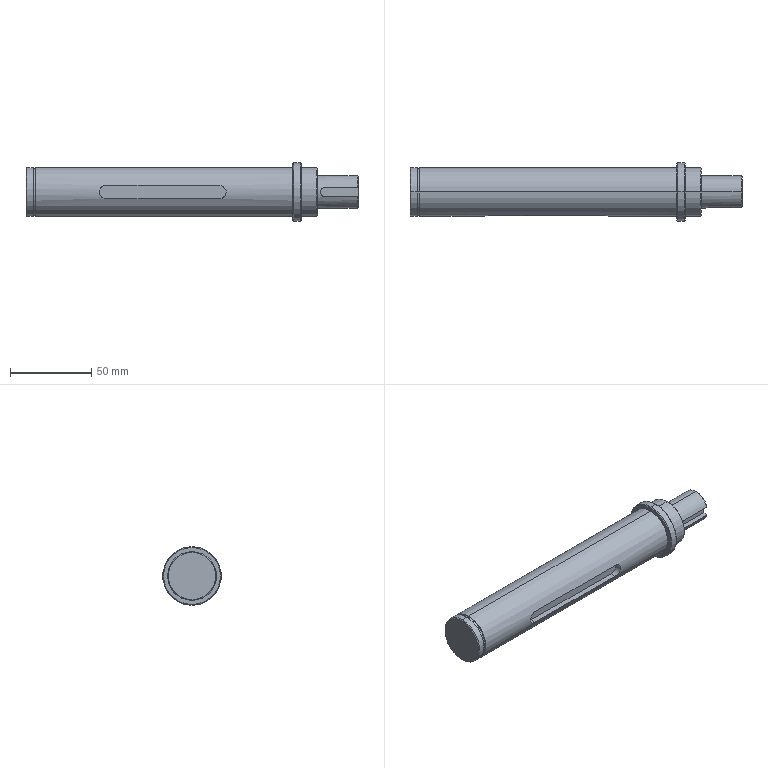Part | SolidWorks | features ICE 2, Chamfer 1, Revolution 1 | 1 solid | 39 faces | box 204 x 36 x 36 mm | volume 132992 mm3 | cylinder 15 | plane 13 | cone 11 | commonest cylinder face diameters 30 x6 8 x2 20 x2 28.6 x2 36 x2 6 x1
STEP:
#1=CARTESIAN_POINT('',(0.,0.,14.5));
#2=VERTEX_POINT('',#1);
#3=CARTESIAN_POINT('',(0.,0.,-14.5));
#4=VERTEX_POINT('',#3);
#5=CARTESIAN_POINT('',(0.,0.,0.));
#6=DIRECTION('',(-1.,0.,0.));
#7=DIRECTION('',(0.,0.,-1.));
#8=AXIS2_PLACEMENT_3D('',#5,#6,#7);
#9=CIRCLE('',#8,14.5);
#10=EDGE_CURVE('',#2,#4,#9,.T.);
#11=ORIENTED_EDGE('',*,*,#10,.F.);
#12=CARTESIAN_POINT('',(0.5,0.,15.));
#13=VERTEX_POINT('',#12);
#14=CARTESIAN_POINT('',(0.,0.,14.5));
#15=DIRECTION('',(0.7071,0.,0.7071));
#16=VECTOR('',#15,1000.);
#17=LINE('',#14,#16);
#18=EDGE_CURVE('',#2,#13,#17,.T.);
#19=ORIENTED_EDGE('',*,*,#18,.T.);
#20=CARTESIAN_POINT('',(0.5,0.,-15.));
#21=VERTEX_POINT('',#20);
#22=CARTESIAN_POINT('',(0.5,0.,0.));
#23=DIRECTION('',(1.,0.,0.));
#24=DIRECTION('',(0.,0.,-1.));
#25=AXIS2_PLACEMENT_3D('',#22,#23,#24);
#26=CIRCLE('',#25,15.);
#27=EDGE_CURVE('',#21,#13,#26,.T.);
#28=ORIENTED_EDGE('',*,*,#27,.F.);
#29=CARTESIAN_POINT('',(0.,0.,-14.5));
#30=DIRECTION('',(0.7071,0.,-0.7071));
#31=VECTOR('',#30,1000.);
#32=LINE('',#29,#31);
#33=EDGE_CURVE('',#4,#21,#32,.T.);
#34=ORIENTED_EDGE('',*,*,#33,.F.);
#35=EDGE_LOOP('',(#11,#19,#28,#34));
#36=FACE_OUTER_BOUND('',#35,.T.);
#37=CARTESIAN_POINT('',(0.,0.,0.));
#38=DIRECTION('',(1.,0.,0.));
#39=DIRECTION('',(0.,0.,-1.));
#40=AXIS2_PLACEMENT_3D('',#37,#38,#39);
#41=CONICAL_SURFACE('',#40,14.5,0.7854);
#42=ADVANCED_FACE('',(#36),#41,.T.);
#43=CARTESIAN_POINT('',(169.,0.,-17.5));
#44=VERTEX_POINT('',#43);
#45=CARTESIAN_POINT('',(169.,0.,17.5));
#46=VERTEX_POINT('',#45);
#47=CARTESIAN_POINT('',(169.,0.,0.));
#48=DIRECTION('',(1.,0.,0.));
#49=DIRECTION('',(0.,0.,1.));
#50=AXIS2_PLACEMENT_3D('',#47,#48,#49);
#51=CIRCLE('',#50,17.5);
#52=EDGE_CURVE('',#44,#46,#51,.T.);
#53=ORIENTED_EDGE('',*,*,#52,.F.);
#54=CARTESIAN_POINT('',(168.5,0.,-18.));
#55=VERTEX_POINT('',#54);
#56=CARTESIAN_POINT('',(168.5,0.,-18.));
#57=DIRECTION('',(-0.7071,0.,-0.7071));
#58=VECTOR('',#57,1000.);
#59=LINE('',#56,#58);
#60=EDGE_CURVE('',#44,#55,#59,.T.);
#61=ORIENTED_EDGE('',*,*,#60,.T.);
#62=CARTESIAN_POINT('',(168.5,0.,18.));
#63=VERTEX_POINT('',#62);
#64=CARTESIAN_POINT('',(168.5,0.,0.));
#65=DIRECTION('',(-1.,0.,0.));
#66=DIRECTION('',(0.,0.,1.));
#67=AXIS2_PLACEMENT_3D('',#64,#65,#66);
#68=CIRCLE('',#67,18.);
#69=EDGE_CURVE('',#63,#55,#68,.T.);
#70=ORIENTED_EDGE('',*,*,#69,.F.);
#71=CARTESIAN_POINT('',(168.5,0.,18.));
#72=DIRECTION('',(-0.7071,0.,0.7071));
#73=VECTOR('',#72,1000.);
#74=LINE('',#71,#73);
#75=EDGE_CURVE('',#46,#63,#74,.T.);
#76=ORIENTED_EDGE('',*,*,#75,.F.);
#77=EDGE_LOOP('',(#53,#61,#70,#76));
#78=FACE_OUTER_BOUND('',#77,.T.);
#79=CARTESIAN_POINT('',(168.5,0.,0.));
#80=DIRECTION('',(-1.,0.,0.));
#81=DIRECTION('',(0.,0.,1.));
#82=AXIS2_PLACEMENT_3D('',#79,#80,#81);
#83=CONICAL_SURFACE('',#82,18.,0.7854);
#84=ADVANCED_FACE('',(#78),#83,.T.);
#85=CARTESIAN_POINT('',(164.,0.,17.5));
#86=VERTEX_POINT('',#85);
#87=CARTESIAN_POINT('',(164.,0.,-17.5));
#88=VERTEX_POINT('',#87);
#89=CARTESIAN_POINT('',(164.,0.,0.));
#90=DIRECTION('',(-1.,0.,0.));
#91=DIRECTION('',(0.,0.,-1.));
#92=AXIS2_PLACEMENT_3D('',#89,#90,#91);
#93=CIRCLE('',#92,17.5);
#94=EDGE_CURVE('',#86,#88,#93,.T.);
#95=ORIENTED_EDGE('',*,*,#94,.F.);
#96=CARTESIAN_POINT('',(164.5,0.,18.));
#97=VERTEX_POINT('',#96);
#98=CARTESIAN_POINT('',(164.,0.,17.5));
#99=DIRECTION('',(0.7071,0.,0.7071));
#100=VECTOR('',#99,1000.);
#101=LINE('',#98,#100);
#102=EDGE_CURVE('',#86,#97,#101,.T.);
#103=ORIENTED_EDGE('',*,*,#102,.T.);
#104=CARTESIAN_POINT('',(164.5,0.,-18.));
#105=VERTEX_POINT('',#104);
#106=CARTESIAN_POINT('',(164.5,0.,0.));
#107=DIRECTION('',(1.,0.,0.));
#108=DIRECTION('',(0.,0.,-1.));
#109=AXIS2_PLACEMENT_3D('',#106,#107,#108);
#110=CIRCLE('',#109,18.);
#111=EDGE_CURVE('',#105,#97,#110,.T.);
#112=ORIENTED_EDGE('',*,*,#111,.F.);
#113=CARTESIAN_POINT('',(164.,0.,-17.5));
#114=DIRECTION('',(0.7071,0.,-0.7071));
#115=VECTOR('',#114,1000.);
#116=LINE('',#113,#115);
#117=EDGE_CURVE('',#88,#105,#116,.T.);
#118=ORIENTED_EDGE('',*,*,#117,.F.);
#119=EDGE_LOOP('',(#95,#103,#112,#118));
#120=FACE_OUTER_BOUND('',#119,.T.);
#121=CARTESIAN_POINT('',(164.,0.,0.));
#122=DIRECTION('',(1.,0.,0.));
#123=DIRECTION('',(0.,0.,-1.));
#124=AXIS2_PLACEMENT_3D('',#121,#122,#123);
#125=CONICAL_SURFACE('',#124,17.5,0.7854);
#126=ADVANCED_FACE('',(#120),#125,.T.);
#127=CARTESIAN_POINT('',(179.,0.,-14.5));
#128=VERTEX_POINT('',#127);
#129=CARTESIAN_POINT('',(179.,0.,14.5));
#130=VERTEX_POINT('',#129);
#131=CARTESIAN_POINT('',(179.,0.,0.));
#132=DIRECTION('',(1.,0.,0.));
#133=DIRECTION('',(0.,0.,1.));
#134=AXIS2_PLACEMENT_3D('',#131,#132,#133);
#135=CIRCLE('',#134,14.5);
#136=EDGE_CURVE('',#128,#130,#135,.T.);
#137=ORIENTED_EDGE('',*,*,#136,.F.);
#138=CARTESIAN_POINT('',(178.5,0.,-15.));
#139=VERTEX_POINT('',#138);
#140=CARTESIAN_POINT('',(178.5,0.,-15.));
#141=DIRECTION('',(-0.7071,0.,-0.7071));
#142=VECTOR('',#141,1000.);
#143=LINE('',#140,#142);
#144=EDGE_CURVE('',#128,#139,#143,.T.);
#145=ORIENTED_EDGE('',*,*,#144,.T.);
#146=CARTESIAN_POINT('',(178.5,0.,15.));
#147=VERTEX_POINT('',#146);
#148=CARTESIAN_POINT('',(178.5,0.,0.));
#149=DIRECTION('',(-1.,0.,0.));
#150=DIRECTION('',(0.,0.,1.));
#151=AXIS2_PLACEMENT_3D('',#148,#149,#150);
#152=CIRCLE('',#151,15.);
#153=EDGE_CURVE('',#147,#139,#152,.T.);
#154=ORIENTED_EDGE('',*,*,#153,.F.);
#155=CARTESIAN_POINT('',(178.5,0.,15.));
#156=DIRECTION('',(-0.7071,0.,0.7071));
#157=VECTOR('',#156,1000.);
#158=LINE('',#155,#157);
#159=EDGE_CURVE('',#130,#147,#158,.T.);
#160=ORIENTED_EDGE('',*,*,#159,.F.);
#161=EDGE_LOOP('',(#137,#145,#154,#160));
#162=FACE_OUTER_BOUND('',#161,.T.);
#163=CARTESIAN_POINT('',(178.5,0.,0.));
#164=DIRECTION('',(-1.,0.,0.));
#165=DIRECTION('',(0.,0.,1.));
#166=AXIS2_PLACEMENT_3D('',#163,#164,#165);
#167=CONICAL_SURFACE('',#166,15.,0.7854);
#168=ADVANCED_FACE('',(#162),#167,.T.);
#169=CARTESIAN_POINT('',(204.,0.,-9.5));
#170=VERTEX_POINT('',#169);
#171=CARTESIAN_POINT('',(204.,0.,9.5));
#172=VERTEX_POINT('',#171);
#173=CARTESIAN_POINT('',(204.,0.,0.));
#174=DIRECTION('',(1.,0.,0.));
#175=DIRECTION('',(0.,0.,1.));
#176=AXIS2_PLACEMENT_3D('',#173,#174,#175);
#177=CIRCLE('',#176,9.5);
#178=EDGE_CURVE('',#170,#172,#177,.T.);
#179=ORIENTED_EDGE('',*,*,#178,.F.);
#180=CARTESIAN_POINT('',(203.5,0.,-10.));
#181=VERTEX_POINT('',#180);
#182=CARTESIAN_POINT('',(203.5,0.,-10.));
#183=DIRECTION('',(-0.7071,0.,-0.7071));
#184=VECTOR('',#183,1000.);
#185=LINE('',#182,#184);
#186=EDGE_CURVE('',#170,#181,#185,.T.);
#187=ORIENTED_EDGE('',*,*,#186,.T.);
#188=CARTESIAN_POINT('',(203.5,0.,10.));
#189=VERTEX_POINT('',#188);
#190=CARTESIAN_POINT('',(203.5,0.,0.));
#191=DIRECTION('',(-1.,0.,0.));
#192=DIRECTION('',(0.,0.,1.));
#193=AXIS2_PLACEMENT_3D('',#190,#191,#192);
#194=CIRCLE('',#193,10.);
#195=EDGE_CURVE('',#189,#181,#194,.T.);
#196=ORIENTED_EDGE('',*,*,#195,.F.);
#197=CARTESIAN_POINT('',(203.5,0.,10.));
#198=DIRECTION('',(-0.7071,0.,0.7071));
#199=VECTOR('',#198,1000.);
#200=LINE('',#197,#199);
#201=EDGE_CURVE('',#172,#189,#200,.T.);
#202=ORIENTED_EDGE('',*,*,#201,.F.);
#203=EDGE_LOOP('',(#179,#187,#196,#202));
#204=FACE_OUTER_BOUND('',#203,.T.);
#205=CARTESIAN_POINT('',(203.5,0.,0.));
#206=DIRECTION('',(-1.,0.,0.));
#207=DIRECTION('',(0.,0.,1.));
#208=AXIS2_PLACEMENT_3D('',#205,#206,#207);
#209=CONICAL_SURFACE('',#208,10.,0.7854);
#210=ADVANCED_FACE('',(#204),#209,.T.);
#211=CARTESIAN_POINT('',(204.,-9.014,3.));
#212=VERTEX_POINT('',#211);
#213=CARTESIAN_POINT('',(204.,0.,0.));
#214=DIRECTION('',(1.,0.,0.));
#215=DIRECTION('',(0.,0.,1.));
#216=AXIS2_PLACEMENT_3D('',#213,#214,#215);
#217=CIRCLE('',#216,9.5);
#218=EDGE_CURVE('',#172,#212,#217,.T.);
#219=ORIENTED_EDGE('',*,*,#218,.F.);
#220=ORIENTED_EDGE('',*,*,#201,.T.);
#221=CARTESIAN_POINT('',(203.5,-9.539,3.));
#222=VERTEX_POINT('',#221);
#223=CARTESIAN_POINT('',(203.5,0.,0.));
#224=DIRECTION('',(-1.,0.,0.));
#225=DIRECTION('',(0.,0.,1.));
#226=AXIS2_PLACEMENT_3D('',#223,#224,#225);
#227=CIRCLE('',#226,10.);
#228=EDGE_CURVE('',#222,#189,#227,.T.);
#229=ORIENTED_EDGE('',*,*,#228,.F.);
#230=CARTESIAN_POINT('',(204.,-9.014,3.));
#231=CARTESIAN_POINT('',(203.834,-9.189,3.));
#232=CARTESIAN_POINT('',(203.667,-9.364,3.));
#233=CARTESIAN_POINT('',(203.5,-9.539,3.));
#234=B_SPLINE_CURVE_WITH_KNOTS('',3,(#230,#231,#232,#233),.UNSPECIFIED.,.F.,.F.,(4,4),(0.005234,0.005959),.UNSPECIFIED.);
#235=EDGE_CURVE('',#212,#222,#234,.T.);
#236=ORIENTED_EDGE('',*,*,#235,.F.);
#237=EDGE_LOOP('',(#219,#220,#229,#236));
#238=FACE_OUTER_BOUND('',#237,.T.);
#239=CARTESIAN_POINT('',(203.5,0.,0.));
#240=DIRECTION('',(-1.,0.,0.));
#241=DIRECTION('',(0.,0.,1.));
#242=AXIS2_PLACEMENT_3D('',#239,#240,#241);
#243=CONICAL_SURFACE('',#242,10.,0.7854);
#244=ADVANCED_FACE('',(#238),#243,.T.);
#245=ORIENTED_EDGE('',*,*,#195,.T.);
#246=CARTESIAN_POINT('',(179.,0.,-10.));
#247=VERTEX_POINT('',#246);
#248=CARTESIAN_POINT('',(0.,0.,-10.));
#249=DIRECTION('',(-1.,0.,0.));
#250=VECTOR('',#249,1000.);
#251=LINE('',#248,#250);
#252=EDGE_CURVE('',#181,#247,#251,.T.);
#253=ORIENTED_EDGE('',*,*,#252,.T.);
#254=CARTESIAN_POINT('',(179.,0.,10.));
#255=VERTEX_POINT('',#254);
#256=CARTESIAN_POINT('',(179.,0.,0.));
#257=DIRECTION('',(-1.,0.,0.));
#258=DIRECTION('',(0.,0.,1.));
#259=AXIS2_PLACEMENT_3D('',#256,#257,#258);
#260=CIRCLE('',#259,10.);
#261=EDGE_CURVE('',#255,#247,#260,.T.);
#262=ORIENTED_EDGE('',*,*,#261,.F.);
#263=CARTESIAN_POINT('',(0.,0.,10.));
#264=DIRECTION('',(-1.,0.,0.));
#265=VECTOR('',#264,1000.);
#266=LINE('',#263,#265);
#267=EDGE_CURVE('',#189,#255,#266,.T.);
#268=ORIENTED_EDGE('',*,*,#267,.F.);
#269=EDGE_LOOP('',(#245,#253,#262,#268));
#270=FACE_OUTER_BOUND('',#269,.T.);
#271=CARTESIAN_POINT('',(0.,0.,0.));
#272=DIRECTION('',(-1.,0.,0.));
#273=DIRECTION('',(0.,0.,1.));
#274=AXIS2_PLACEMENT_3D('',#271,#272,#273);
#275=CYLINDRICAL_SURFACE('',#274,10.);
#276=ADVANCED_FACE('',(#270),#275,.T.);
#277=ORIENTED_EDGE('',*,*,#153,.T.);
#278=CARTESIAN_POINT('',(169.,0.,-15.));
#279=VERTEX_POINT('',#278);
#280=CARTESIAN_POINT('',(0.,0.,-15.));
#281=DIRECTION('',(-1.,0.,0.));
#282=VECTOR('',#281,1000.);
#283=LINE('',#280,#282);
#284=EDGE_CURVE('',#139,#279,#283,.T.);
#285=ORIENTED_EDGE('',*,*,#284,.T.);
#286=CARTESIAN_POINT('',(169.,0.,15.));
#287=VERTEX_POINT('',#286);
#288=CARTESIAN_POINT('',(169.,0.,0.));
#289=DIRECTION('',(-1.,0.,0.));
#290=DIRECTION('',(0.,0.,1.));
#291=AXIS2_PLACEMENT_3D('',#288,#289,#290);
#292=CIRCLE('',#291,15.);
#293=EDGE_CURVE('',#287,#279,#292,.T.);
#294=ORIENTED_EDGE('',*,*,#293,.F.);
#295=CARTESIAN_POINT('',(0.,0.,15.));
#296=DIRECTION('',(-1.,0.,0.));
#297=VECTOR('',#296,1000.);
#298=LINE('',#295,#297);
#299=EDGE_CURVE('',#147,#287,#298,.T.);
#300=ORIENTED_EDGE('',*,*,#299,.F.);
#301=EDGE_LOOP('',(#277,#285,#294,#300));
#302=FACE_OUTER_BOUND('',#301,.T.);
#303=CARTESIAN_POINT('',(0.,0.,0.));
#304=DIRECTION('',(-1.,0.,0.));
#305=DIRECTION('',(0.,0.,1.));
#306=AXIS2_PLACEMENT_3D('',#303,#304,#305);
#307=CYLINDRICAL_SURFACE('',#306,15.);
#308=ADVANCED_FACE('',(#302),#307,.T.);
#309=ORIENTED_EDGE('',*,*,#69,.T.);
#310=CARTESIAN_POINT('',(0.,0.,-18.));
#311=DIRECTION('',(-1.,0.,0.));
#312=VECTOR('',#311,1000.);
#313=LINE('',#310,#312);
#314=EDGE_CURVE('',#55,#105,#313,.T.);
#315=ORIENTED_EDGE('',*,*,#314,.T.);
#316=ORIENTED_EDGE('',*,*,#111,.T.);
#317=CARTESIAN_POINT('',(0.,0.,18.));
#318=DIRECTION('',(-1.,0.,0.));
#319=VECTOR('',#318,1000.);
#320=LINE('',#317,#319);
#321=EDGE_CURVE('',#63,#97,#320,.T.);
#322=ORIENTED_EDGE('',*,*,#321,.F.);
#323=EDGE_LOOP('',(#309,#315,#316,#322));
#324=FACE_OUTER_BOUND('',#323,.T.);
#325=CARTESIAN_POINT('',(0.,0.,0.));
#326=DIRECTION('',(-1.,0.,0.));
#327=DIRECTION('',(0.,0.,1.));
#328=AXIS2_PLACEMENT_3D('',#325,#326,#327);
#329=CYLINDRICAL_SURFACE('',#328,18.);
#330=ADVANCED_FACE('',(#324),#329,.T.);
#331=CARTESIAN_POINT('',(164.,0.,15.));
#332=VERTEX_POINT('',#331);
#333=CARTESIAN_POINT('',(164.,0.,-15.));
#334=VERTEX_POINT('',#333);
#335=CARTESIAN_POINT('',(164.,0.,0.));
#336=DIRECTION('',(-1.,0.,0.));
#337=DIRECTION('',(0.,0.,1.));
#338=AXIS2_PLACEMENT_3D('',#335,#336,#337);
#339=CIRCLE('',#338,15.);
#340=EDGE_CURVE('',#332,#334,#339,.T.);
#341=ORIENTED_EDGE('',*,*,#340,.T.);
#342=CARTESIAN_POINT('',(6.,0.,-15.));
#343=VERTEX_POINT('',#342);
#344=CARTESIAN_POINT('',(0.,0.,-15.));
#345=DIRECTION('',(-1.,0.,0.));
#346=VECTOR('',#345,1000.);
#347=LINE('',#344,#346);
#348=EDGE_CURVE('',#334,#343,#347,.T.);
#349=ORIENTED_EDGE('',*,*,#348,.T.);
#350=CARTESIAN_POINT('',(6.,0.,15.));
#351=VERTEX_POINT('',#350);
#352=CARTESIAN_POINT('',(6.,0.,0.));
#353=DIRECTION('',(-1.,0.,0.));
#354=DIRECTION('',(0.,0.,1.));
#355=AXIS2_PLACEMENT_3D('',#352,#353,#354);
#356=CIRCLE('',#355,15.);
#357=EDGE_CURVE('',#351,#343,#356,.T.);
#358=ORIENTED_EDGE('',*,*,#357,.F.);
#359=CARTESIAN_POINT('',(0.,0.,15.));
#360=DIRECTION('',(-1.,0.,0.));
#361=VECTOR('',#360,1000.);
#362=LINE('',#359,#361);
#363=EDGE_CURVE('',#332,#351,#362,.T.);
#364=ORIENTED_EDGE('',*,*,#363,.F.);
#365=EDGE_LOOP('',(#341,#349,#358,#364));
#366=FACE_OUTER_BOUND('',#365,.T.);
#367=CARTESIAN_POINT('',(0.,0.,0.));
#368=DIRECTION('',(-1.,0.,0.));
#369=DIRECTION('',(0.,0.,1.));
#370=AXIS2_PLACEMENT_3D('',#367,#368,#369);
#371=CYLINDRICAL_SURFACE('',#370,15.);
#372=ADVANCED_FACE('',(#366),#371,.T.);
#373=CARTESIAN_POINT('',(6.,0.,14.3));
#374=VERTEX_POINT('',#373);
#375=CARTESIAN_POINT('',(6.,0.,-14.3));
#376=VERTEX_POINT('',#375);
#377=CARTESIAN_POINT('',(6.,0.,0.));
#378=DIRECTION('',(-1.,0.,0.));
#379=DIRECTION('',(0.,0.,1.));
#380=AXIS2_PLACEMENT_3D('',#377,#378,#379);
#381=CIRCLE('',#380,14.3);
#382=EDGE_CURVE('',#374,#376,#381,.T.);
#383=ORIENTED_EDGE('',*,*,#382,.T.);
#384=CARTESIAN_POINT('',(4.4,0.,-14.3));
#385=VERTEX_POINT('',#384);
#386=CARTESIAN_POINT('',(0.,0.,-14.3));
#387=DIRECTION('',(-1.,0.,0.));
#388=VECTOR('',#387,1000.);
#389=LINE('',#386,#388);
#390=EDGE_CURVE('',#376,#385,#389,.T.);
#391=ORIENTED_EDGE('',*,*,#390,.T.);
#392=CARTESIAN_POINT('',(4.4,0.,14.3));
#393=VERTEX_POINT('',#392);
#394=CARTESIAN_POINT('',(4.4,0.,0.));
#395=DIRECTION('',(-1.,0.,0.));
#396=DIRECTION('',(0.,0.,1.));
#397=AXIS2_PLACEMENT_3D('',#394,#395,#396);
#398=CIRCLE('',#397,14.3);
#399=EDGE_CURVE('',#393,#385,#398,.T.);
#400=ORIENTED_EDGE('',*,*,#399,.F.);
#401=CARTESIAN_POINT('',(0.,0.,14.3));
#402=DIRECTION('',(-1.,0.,0.));
#403=VECTOR('',#402,1000.);
#404=LINE('',#401,#403);
#405=EDGE_CURVE('',#374,#393,#404,.T.);
#406=ORIENTED_EDGE('',*,*,#405,.F.);
#407=EDGE_LOOP('',(#383,#391,#400,#406));
#408=FACE_OUTER_BOUND('',#407,.T.);
#409=CARTESIAN_POINT('',(0.,0.,0.));
#410=DIRECTION('',(-1.,0.,0.));
#411=DIRECTION('',(0.,0.,1.));
#412=AXIS2_PLACEMENT_3D('',#409,#410,#411);
#413=CYLINDRICAL_SURFACE('',#412,14.3);
#414=ADVANCED_FACE('',(#408),#413,.T.);
#415=CARTESIAN_POINT('',(4.4,0.,15.));
#416=VERTEX_POINT('',#415);
#417=CARTESIAN_POINT('',(4.4,0.,-15.));
#418=VERTEX_POINT('',#417);
#419=CARTESIAN_POINT('',(4.4,0.,0.));
#420=DIRECTION('',(-1.,0.,0.));
#421=DIRECTION('',(0.,0.,1.));
#422=AXIS2_PLACEMENT_3D('',#419,#420,#421);
#423=CIRCLE('',#422,15.);
#424=EDGE_CURVE('',#416,#418,#423,.T.);
#425=ORIENTED_EDGE('',*,*,#424,.T.);
#426=CARTESIAN_POINT('',(0.,0.,-15.));
#427=DIRECTION('',(-1.,0.,0.));
#428=VECTOR('',#427,1000.);
#429=LINE('',#426,#428);
#430=EDGE_CURVE('',#418,#21,#429,.T.);
#431=ORIENTED_EDGE('',*,*,#430,.T.);
#432=ORIENTED_EDGE('',*,*,#27,.T.);
#433=CARTESIAN_POINT('',(0.,0.,15.));
#434=DIRECTION('',(-1.,0.,0.));
#435=VECTOR('',#434,1000.);
#436=LINE('',#433,#435);
#437=EDGE_CURVE('',#416,#13,#436,.T.);
#438=ORIENTED_EDGE('',*,*,#437,.F.);
#439=EDGE_LOOP('',(#425,#431,#432,#438));
#440=FACE_OUTER_BOUND('',#439,.T.);
#441=CARTESIAN_POINT('',(0.,0.,0.));
#442=DIRECTION('',(-1.,0.,0.));
#443=DIRECTION('',(0.,0.,1.));
#444=AXIS2_PLACEMENT_3D('',#441,#442,#443);
#445=CYLINDRICAL_SURFACE('',#444,15.);
#446=ADVANCED_FACE('',(#440),#445,.T.);
#447=CARTESIAN_POINT('',(0.,0.,0.));
#448=DIRECTION('',(-1.,0.,0.));
#449=DIRECTION('',(0.,0.,-1.));
#450=AXIS2_PLACEMENT_3D('',#447,#448,#449);
#451=CIRCLE('',#450,14.5);
#452=EDGE_CURVE('',#4,#2,#451,.T.);
#453=ORIENTED_EDGE('',*,*,#452,.T.);
#454=ORIENTED_EDGE('',*,*,#10,.T.);
#455=EDGE_LOOP('',(#453,#454));
#456=FACE_OUTER_BOUND('',#455,.T.);
#457=CARTESIAN_POINT('',(0.,0.,0.));
#458=DIRECTION('',(1.,0.,0.));
#459=DIRECTION('',(0.,0.,-1.));
#460=AXIS2_PLACEMENT_3D('',#457,#458,#459);
#461=PLANE('',#460);
#462=ADVANCED_FACE('',(#456),#461,.F.);
#463=ORIENTED_EDGE('',*,*,#430,.F.);
#464=CARTESIAN_POINT('',(4.4,0.,0.));
#465=DIRECTION('',(-1.,0.,0.));
#466=DIRECTION('',(0.,0.,1.));
#467=AXIS2_PLACEMENT_3D('',#464,#465,#466);
#468=CIRCLE('',#467,15.);
#469=EDGE_CURVE('',#418,#416,#468,.T.);
#470=ORIENTED_EDGE('',*,*,#469,.T.);
#471=ORIENTED_EDGE('',*,*,#437,.T.);
#472=CARTESIAN_POINT('',(0.5,0.,0.));
#473=DIRECTION('',(1.,0.,0.));
#474=DIRECTION('',(0.,0.,-1.));
#475=AXIS2_PLACEMENT_3D('',#472,#473,#474);
#476=CIRCLE('',#475,15.);
#477=EDGE_CURVE('',#13,#21,#476,.T.);
#478=ORIENTED_EDGE('',*,*,#477,.T.);
#479=EDGE_LOOP('',(#463,#470,#471,#478));
#480=FACE_OUTER_BOUND('',#479,.T.);
#481=CARTESIAN_POINT('',(0.,0.,0.));
#482=DIRECTION('',(-1.,0.,0.));
#483=DIRECTION('',(0.,0.,1.));
#484=AXIS2_PLACEMENT_3D('',#481,#482,#483);
#485=CYLINDRICAL_SURFACE('',#484,15.);
#486=ADVANCED_FACE('',(#480),#485,.T.);
#487=ORIENTED_EDGE('',*,*,#424,.F.);
#488=ORIENTED_EDGE('',*,*,#469,.F.);
#489=EDGE_LOOP('',(#487,#488));
#490=FACE_OUTER_BOUND('',#489,.T.);
#491=ORIENTED_EDGE('',*,*,#399,.T.);
#492=CARTESIAN_POINT('',(4.4,0.,0.));
#493=DIRECTION('',(-1.,0.,0.));
#494=DIRECTION('',(0.,0.,1.));
#495=AXIS2_PLACEMENT_3D('',#492,#493,#494);
#496=CIRCLE('',#495,14.3);
#497=EDGE_CURVE('',#385,#393,#496,.T.);
#498=ORIENTED_EDGE('',*,*,#497,.T.);
#499=EDGE_LOOP('',(#491,#498));
#500=FACE_BOUND('',#499,.T.);
#501=CARTESIAN_POINT('',(4.4,15.,0.));
#502=DIRECTION('',(-1.,0.,0.));
#503=DIRECTION('',(0.,0.,1.));
#504=AXIS2_PLACEMENT_3D('',#501,#502,#503);
#505=PLANE('',#504);
#506=ADVANCED_FACE('',(#490,#500),#505,.F.);
#507=ORIENTED_EDGE('',*,*,#390,.F.);
#508=CARTESIAN_POINT('',(6.,0.,0.));
#509=DIRECTION('',(-1.,0.,0.));
#510=DIRECTION('',(0.,0.,1.));
#511=AXIS2_PLACEMENT_3D('',#508,#509,#510);
#512=CIRCLE('',#511,14.3);
#513=EDGE_CURVE('',#376,#374,#512,.T.);
#514=ORIENTED_EDGE('',*,*,#513,.T.);
#515=ORIENTED_EDGE('',*,*,#405,.T.);
#516=ORIENTED_EDGE('',*,*,#497,.F.);
#517=EDGE_LOOP('',(#507,#514,#515,#516));
#518=FACE_OUTER_BOUND('',#517,.T.);
#519=CARTESIAN_POINT('',(0.,0.,0.));
#520=DIRECTION('',(-1.,0.,0.));
#521=DIRECTION('',(0.,0.,1.));
#522=AXIS2_PLACEMENT_3D('',#519,#520,#521);
#523=CYLINDRICAL_SURFACE('',#522,14.3);
#524=ADVANCED_FACE('',(#518),#523,.T.);
#525=ORIENTED_EDGE('',*,*,#382,.F.);
#526=ORIENTED_EDGE('',*,*,#513,.F.);
#527=EDGE_LOOP('',(#525,#526));
#528=FACE_BOUND('',#527,.T.);
#529=ORIENTED_EDGE('',*,*,#357,.T.);
#530=CARTESIAN_POINT('',(6.,0.,0.));
#531=DIRECTION('',(-1.,0.,0.));
#532=DIRECTION('',(0.,0.,1.));
#533=AXIS2_PLACEMENT_3D('',#530,#531,#532);
#534=CIRCLE('',#533,15.);
#535=EDGE_CURVE('',#343,#351,#534,.T.);
#536=ORIENTED_EDGE('',*,*,#535,.T.);
#537=EDGE_LOOP('',(#529,#536));
#538=FACE_OUTER_BOUND('',#537,.T.);
#539=CARTESIAN_POINT('',(6.,14.3,0.));
#540=DIRECTION('',(1.,0.,0.));
#541=DIRECTION('',(0.,0.,-1.));
#542=AXIS2_PLACEMENT_3D('',#539,#540,#541);
#543=PLANE('',#542);
#544=ADVANCED_FACE('',(#528,#538),#543,.F.);
#545=ORIENTED_EDGE('',*,*,#348,.F.);
#546=CARTESIAN_POINT('',(164.,0.,0.));
#547=DIRECTION('',(-1.,0.,0.));
#548=DIRECTION('',(0.,0.,1.));
#549=AXIS2_PLACEMENT_3D('',#546,#547,#548);
#550=CIRCLE('',#549,15.);
#551=EDGE_CURVE('',#334,#332,#550,.T.);
#552=ORIENTED_EDGE('',*,*,#551,.T.);
#553=ORIENTED_EDGE('',*,*,#363,.T.);
#554=ORIENTED_EDGE('',*,*,#535,.F.);
#555=EDGE_LOOP('',(#545,#552,#553,#554));
#556=FACE_OUTER_BOUND('',#555,.T.);
#557=CARTESIAN_POINT('',(49.,-14.457,4.));
#558=VERTEX_POINT('',#557);
#559=CARTESIAN_POINT('',(119.,-14.457,4.));
#560=VERTEX_POINT('',#559);
#561=CARTESIAN_POINT('',(0.,-14.457,4.));
#562=DIRECTION('',(1.,0.,0.));
#563=VECTOR('',#562,1000.);
#564=LINE('',#561,#563);
#565=EDGE_CURVE('',#558,#560,#564,.T.);
#566=ORIENTED_EDGE('',*,*,#565,.T.);
#567=CARTESIAN_POINT('',(119.,-14.457,-4.));
#568=VERTEX_POINT('',#567);
#569=CARTESIAN_POINT('',(119.,-14.457,4.));
#570=CARTESIAN_POINT('',(119.266,-14.457,4.));
#571=CARTESIAN_POINT('',(119.526,-14.464,3.974));
#572=CARTESIAN_POINT('',(120.039,-14.492,3.872));
#573=CARTESIAN_POINT('',(120.294,-14.513,3.794));
#574=CARTESIAN_POINT('',(120.777,-14.564,3.593));
#575=CARTESIAN_POINT('',(121.007,-14.594,3.47));
#576=CARTESIAN_POINT('',(121.44,-14.66,3.18));
#577=CARTESIAN_POINT('',(121.645,-14.696,3.012));
#578=CARTESIAN_POINT('',(122.012,-14.766,2.645));
#579=CARTESIAN_POINT('',(122.177,-14.801,2.444));
#580=CARTESIAN_POINT('',(122.47,-14.867,2.008));
#581=CARTESIAN_POINT('',(122.593,-14.896,1.777));
#582=CARTESIAN_POINT('',(122.793,-14.946,1.296));
#583=CARTESIAN_POINT('',(122.871,-14.966,1.043));
#584=CARTESIAN_POINT('',(122.974,-14.993,0.5261));
#585=CARTESIAN_POINT('',(123.,-15.,0.2658));
#586=CARTESIAN_POINT('',(123.,-15.,-0.2585));
#587=CARTESIAN_POINT('',(122.974,-14.993,-0.5249));
#588=CARTESIAN_POINT('',(122.872,-14.966,-1.039));
#589=CARTESIAN_POINT('',(122.796,-14.947,-1.289));
#590=CARTESIAN_POINT('',(122.494,-14.872,-2.017));
#591=CARTESIAN_POINT('',(122.199,-14.802,-2.457));
#592=CARTESIAN_POINT('',(121.645,-14.696,-3.012));
#593=CARTESIAN_POINT('',(121.444,-14.66,-3.177));
#594=CARTESIAN_POINT('',(121.012,-14.595,-3.467));
#595=CARTESIAN_POINT('',(120.778,-14.564,-3.593));
#596=CARTESIAN_POINT('',(120.296,-14.513,-3.793));
#597=CARTESIAN_POINT('',(120.046,-14.492,-3.87));
#598=CARTESIAN_POINT('',(119.531,-14.464,-3.973));
#599=CARTESIAN_POINT('',(119.266,-14.457,-4.));
#600=CARTESIAN_POINT('',(119.,-14.457,-4.));
#601=B_SPLINE_CURVE_WITH_KNOTS('',3,(#569,#570,#571,#572,#573,#574,#575,#576,#577,#578,#579,#580,#581,#582,#583,#584,#585,#586,#587,#588,#589,#590,#591,#592,#593,#594,#595,#596,#597,#598,#599,#600),.UNSPECIFIED.,.F.,.F.,(4,2,2,2,2,2,2,2,2,2,2,2,2,2,2,4),(0.,0.0007849,0.00157,0.002355,0.00314,0.003925,0.00471,0.005494,0.006279,0.007064,0.007849,0.009419,0.0102,0.01099,0.01177,0.01256),.UNSPECIFIED.);
#602=EDGE_CURVE('',#560,#568,#601,.T.);
#603=ORIENTED_EDGE('',*,*,#602,.T.);
#604=CARTESIAN_POINT('',(49.,-14.457,-4.));
#605=VERTEX_POINT('',#604);
#606=CARTESIAN_POINT('',(0.,-14.457,-4.));
#607=DIRECTION('',(-1.,0.,0.));
#608=VECTOR('',#607,1000.);
#609=LINE('',#606,#608);
#610=EDGE_CURVE('',#568,#605,#609,.T.);
#611=ORIENTED_EDGE('',*,*,#610,.T.);
#612=CARTESIAN_POINT('',(49.,-14.457,-4.));
#613=CARTESIAN_POINT('',(48.734,-14.457,-4.));
#614=CARTESIAN_POINT('',(48.474,-14.464,-3.974));
#615=CARTESIAN_POINT('',(47.961,-14.492,-3.872));
#616=CARTESIAN_POINT('',(47.706,-14.513,-3.794));
#617=CARTESIAN_POINT('',(47.223,-14.564,-3.593));
#618=CARTESIAN_POINT('',(46.993,-14.594,-3.47));
#619=CARTESIAN_POINT('',(46.56,-14.66,-3.18));
#620=CARTESIAN_POINT('',(46.355,-14.696,-3.012));
#621=CARTESIAN_POINT('',(45.988,-14.766,-2.645));
#622=CARTESIAN_POINT('',(45.823,-14.801,-2.444));
#623=CARTESIAN_POINT('',(45.53,-14.867,-2.008));
#624=CARTESIAN_POINT('',(45.407,-14.896,-1.777));
#625=CARTESIAN_POINT('',(45.207,-14.946,-1.296));
#626=CARTESIAN_POINT('',(45.129,-14.966,-1.043));
#627=CARTESIAN_POINT('',(45.026,-14.993,-0.5261));
#628=CARTESIAN_POINT('',(45.,-15.,-0.2658));
#629=CARTESIAN_POINT('',(45.,-15.,0.2585));
#630=CARTESIAN_POINT('',(45.026,-14.993,0.5249));
#631=CARTESIAN_POINT('',(45.128,-14.966,1.039));
#632=CARTESIAN_POINT('',(45.204,-14.947,1.289));
#633=CARTESIAN_POINT('',(45.506,-14.872,2.017));
#634=CARTESIAN_POINT('',(45.801,-14.802,2.457));
#635=CARTESIAN_POINT('',(46.355,-14.696,3.012));
#636=CARTESIAN_POINT('',(46.556,-14.66,3.177));
#637=CARTESIAN_POINT('',(46.988,-14.595,3.467));
#638=CARTESIAN_POINT('',(47.222,-14.564,3.593));
#639=CARTESIAN_POINT('',(47.704,-14.513,3.793));
#640=CARTESIAN_POINT('',(47.954,-14.492,3.87));
#641=CARTESIAN_POINT('',(48.469,-14.464,3.973));
#642=CARTESIAN_POINT('',(48.734,-14.457,4.));
#643=CARTESIAN_POINT('',(49.,-14.457,4.));
#644=B_SPLINE_CURVE_WITH_KNOTS('',3,(#612,#613,#614,#615,#616,#617,#618,#619,#620,#621,#622,#623,#624,#625,#626,#627,#628,#629,#630,#631,#632,#633,#634,#635,#636,#637,#638,#639,#640,#641,#642,#643),.UNSPECIFIED.,.F.,.F.,(4,2,2,2,2,2,2,2,2,2,2,2,2,2,2,4),(0.,0.0007849,0.00157,0.002355,0.00314,0.003925,0.00471,0.005494,0.006279,0.007064,0.007849,0.009419,0.0102,0.01099,0.01177,0.01256),.UNSPECIFIED.);
#645=EDGE_CURVE('',#605,#558,#644,.T.);
#646=ORIENTED_EDGE('',*,*,#645,.T.);
#647=EDGE_LOOP('',(#566,#603,#611,#646));
#648=FACE_BOUND('',#647,.T.);
#649=CARTESIAN_POINT('',(0.,0.,0.));
#650=DIRECTION('',(-1.,0.,0.));
#651=DIRECTION('',(0.,0.,1.));
#652=AXIS2_PLACEMENT_3D('',#649,#650,#651);
#653=CYLINDRICAL_SURFACE('',#652,15.);
#654=ADVANCED_FACE('',(#556,#648),#653,.T.);
#655=CARTESIAN_POINT('',(164.,0.,0.));
#656=DIRECTION('',(-1.,0.,0.));
#657=DIRECTION('',(0.,0.,-1.));
#658=AXIS2_PLACEMENT_3D('',#655,#656,#657);
#659=CIRCLE('',#658,17.5);
#660=EDGE_CURVE('',#88,#86,#659,.T.);
#661=ORIENTED_EDGE('',*,*,#660,.T.);
#662=ORIENTED_EDGE('',*,*,#94,.T.);
#663=EDGE_LOOP('',(#661,#662));
#664=FACE_OUTER_BOUND('',#663,.T.);
#665=ORIENTED_EDGE('',*,*,#340,.F.);
#666=ORIENTED_EDGE('',*,*,#551,.F.);
#667=EDGE_LOOP('',(#665,#666));
#668=FACE_BOUND('',#667,.T.);
#669=CARTESIAN_POINT('',(164.,15.,0.));
#670=DIRECTION('',(1.,0.,0.));
#671=DIRECTION('',(0.,0.,-1.));
#672=AXIS2_PLACEMENT_3D('',#669,#670,#671);
#673=PLANE('',#672);
#674=ADVANCED_FACE('',(#664,#668),#673,.F.);
#675=ORIENTED_EDGE('',*,*,#314,.F.);
#676=CARTESIAN_POINT('',(168.5,0.,0.));
#677=DIRECTION('',(-1.,0.,0.));
#678=DIRECTION('',(0.,0.,1.));
#679=AXIS2_PLACEMENT_3D('',#676,#677,#678);
#680=CIRCLE('',#679,18.);
#681=EDGE_CURVE('',#55,#63,#680,.T.);
#682=ORIENTED_EDGE('',*,*,#681,.T.);
#683=ORIENTED_EDGE('',*,*,#321,.T.);
#684=CARTESIAN_POINT('',(164.5,0.,0.));
#685=DIRECTION('',(1.,0.,0.));
#686=DIRECTION('',(0.,0.,-1.));
#687=AXIS2_PLACEMENT_3D('',#684,#685,#686);
#688=CIRCLE('',#687,18.);
#689=EDGE_CURVE('',#97,#105,#688,.T.);
#690=ORIENTED_EDGE('',*,*,#689,.T.);
#691=EDGE_LOOP('',(#675,#682,#683,#690));
#692=FACE_OUTER_BOUND('',#691,.T.);
#693=CARTESIAN_POINT('',(0.,0.,0.));
#694=DIRECTION('',(-1.,0.,0.));
#695=DIRECTION('',(0.,0.,1.));
#696=AXIS2_PLACEMENT_3D('',#693,#694,#695);
#697=CYLINDRICAL_SURFACE('',#696,18.);
#698=ADVANCED_FACE('',(#692),#697,.T.);
#699=CARTESIAN_POINT('',(169.,0.,0.));
#700=DIRECTION('',(1.,0.,0.));
#701=DIRECTION('',(0.,0.,1.));
#702=AXIS2_PLACEMENT_3D('',#699,#700,#701);
#703=CIRCLE('',#702,17.5);
#704=EDGE_CURVE('',#46,#44,#703,.T.);
#705=ORIENTED_EDGE('',*,*,#704,.T.);
#706=ORIENTED_EDGE('',*,*,#52,.T.);
#707=EDGE_LOOP('',(#705,#706));
#708=FACE_OUTER_BOUND('',#707,.T.);
#709=ORIENTED_EDGE('',*,*,#293,.T.);
#710=CARTESIAN_POINT('',(169.,0.,0.));
#711=DIRECTION('',(-1.,0.,0.));
#712=DIRECTION('',(0.,0.,1.));
#713=AXIS2_PLACEMENT_3D('',#710,#711,#712);
#714=CIRCLE('',#713,15.);
#715=EDGE_CURVE('',#279,#287,#714,.T.);
#716=ORIENTED_EDGE('',*,*,#715,.T.);
#717=EDGE_LOOP('',(#709,#716));
#718=FACE_BOUND('',#717,.T.);
#719=CARTESIAN_POINT('',(169.,18.,0.));
#720=DIRECTION('',(-1.,0.,0.));
#721=DIRECTION('',(0.,0.,1.));
#722=AXIS2_PLACEMENT_3D('',#719,#720,#721);
#723=PLANE('',#722);
#724=ADVANCED_FACE('',(#708,#718),#723,.F.);
#725=ORIENTED_EDGE('',*,*,#284,.F.);
#726=CARTESIAN_POINT('',(178.5,0.,0.));
#727=DIRECTION('',(-1.,0.,0.));
#728=DIRECTION('',(0.,0.,1.));
#729=AXIS2_PLACEMENT_3D('',#726,#727,#728);
#730=CIRCLE('',#729,15.);
#731=EDGE_CURVE('',#139,#147,#730,.T.);
#732=ORIENTED_EDGE('',*,*,#731,.T.);
#733=ORIENTED_EDGE('',*,*,#299,.T.);
#734=ORIENTED_EDGE('',*,*,#715,.F.);
#735=EDGE_LOOP('',(#725,#732,#733,#734));
#736=FACE_OUTER_BOUND('',#735,.T.);
#737=CARTESIAN_POINT('',(0.,0.,0.));
#738=DIRECTION('',(-1.,0.,0.));
#739=DIRECTION('',(0.,0.,1.));
#740=AXIS2_PLACEMENT_3D('',#737,#738,#739);
#741=CYLINDRICAL_SURFACE('',#740,15.);
#742=ADVANCED_FACE('',(#736),#741,.T.);
#743=CARTESIAN_POINT('',(179.,0.,0.));
#744=DIRECTION('',(1.,0.,0.));
#745=DIRECTION('',(0.,0.,1.));
#746=AXIS2_PLACEMENT_3D('',#743,#744,#745);
#747=CIRCLE('',#746,14.5);
#748=EDGE_CURVE('',#130,#128,#747,.T.);
#749=ORIENTED_EDGE('',*,*,#748,.T.);
#750=ORIENTED_EDGE('',*,*,#136,.T.);
#751=EDGE_LOOP('',(#749,#750));
#752=FACE_OUTER_BOUND('',#751,.T.);
#753=ORIENTED_EDGE('',*,*,#261,.T.);
#754=CARTESIAN_POINT('',(179.,0.,0.));
#755=DIRECTION('',(-1.,0.,0.));
#756=DIRECTION('',(0.,0.,1.));
#757=AXIS2_PLACEMENT_3D('',#754,#755,#756);
#758=CIRCLE('',#757,10.);
#759=EDGE_CURVE('',#247,#255,#758,.T.);
#760=ORIENTED_EDGE('',*,*,#759,.T.);
#761=EDGE_LOOP('',(#753,#760));
#762=FACE_BOUND('',#761,.T.);
#763=CARTESIAN_POINT('',(179.,15.,0.));
#764=DIRECTION('',(-1.,0.,0.));
#765=DIRECTION('',(0.,0.,1.));
#766=AXIS2_PLACEMENT_3D('',#763,#764,#765);
#767=PLANE('',#766);
#768=ADVANCED_FACE('',(#752,#762),#767,.F.);
#769=ORIENTED_EDGE('',*,*,#252,.F.);
#770=CARTESIAN_POINT('',(203.5,-9.539,-3.));
#771=VERTEX_POINT('',#770);
#772=CARTESIAN_POINT('',(203.5,0.,0.));
#773=DIRECTION('',(-1.,0.,0.));
#774=DIRECTION('',(0.,0.,1.));
#775=AXIS2_PLACEMENT_3D('',#772,#773,#774);
#776=CIRCLE('',#775,10.);
#777=EDGE_CURVE('',#181,#771,#776,.T.);
#778=ORIENTED_EDGE('',*,*,#777,.T.);
#779=CARTESIAN_POINT('',(184.,-9.539,-3.));
#780=VERTEX_POINT('',#779);
#781=CARTESIAN_POINT('',(0.,-9.539,-3.));
#782=DIRECTION('',(-1.,0.,0.));
#783=VECTOR('',#782,1000.);
#784=LINE('',#781,#783);
#785=EDGE_CURVE('',#771,#780,#784,.T.);
#786=ORIENTED_EDGE('',*,*,#785,.T.);
#787=CARTESIAN_POINT('',(184.,-9.539,3.));
#788=VERTEX_POINT('',#787);
#789=CARTESIAN_POINT('',(184.,-9.539,-3.));
#790=CARTESIAN_POINT('',(183.801,-9.539,-3.));
#791=CARTESIAN_POINT('',(183.605,-9.546,-2.98));
#792=CARTESIAN_POINT('',(183.22,-9.569,-2.903));
#793=CARTESIAN_POINT('',(183.029,-9.587,-2.845));
#794=CARTESIAN_POINT('',(182.666,-9.631,-2.694));
#795=CARTESIAN_POINT('',(182.494,-9.656,-2.602));
#796=CARTESIAN_POINT('',(182.169,-9.712,-2.385));
#797=CARTESIAN_POINT('',(182.016,-9.743,-2.259));
#798=CARTESIAN_POINT('',(181.604,-9.832,-1.847));
#799=CARTESIAN_POINT('',(181.381,-9.891,-1.514));
#800=CARTESIAN_POINT('',(181.156,-9.954,-0.9732));
#801=CARTESIAN_POINT('',(181.097,-9.971,-0.783));
#802=CARTESIAN_POINT('',(181.02,-9.994,-0.3953));
#803=CARTESIAN_POINT('',(181.,-10.,-0.1999));
#804=CARTESIAN_POINT('',(181.,-10.,0.194));
#805=CARTESIAN_POINT('',(181.019,-9.994,0.394));
#806=CARTESIAN_POINT('',(181.096,-9.971,0.7797));
#807=CARTESIAN_POINT('',(181.153,-9.955,0.9673));
#808=CARTESIAN_POINT('',(181.305,-9.913,1.332));
#809=CARTESIAN_POINT('',(181.398,-9.887,1.506));
#810=CARTESIAN_POINT('',(181.614,-9.833,1.83));
#811=CARTESIAN_POINT('',(181.74,-9.803,1.982));
#812=CARTESIAN_POINT('',(182.016,-9.743,2.259));
#813=CARTESIAN_POINT('',(182.167,-9.713,2.383));
#814=CARTESIAN_POINT('',(182.49,-9.657,2.6));
#815=CARTESIAN_POINT('',(182.666,-9.631,2.694));
#816=CARTESIAN_POINT('',(183.027,-9.587,2.845));
#817=CARTESIAN_POINT('',(183.214,-9.57,2.902));
#818=CARTESIAN_POINT('',(183.601,-9.546,2.98));
#819=CARTESIAN_POINT('',(183.801,-9.539,3.));
#820=CARTESIAN_POINT('',(184.,-9.539,3.));
#821=B_SPLINE_CURVE_WITH_KNOTS('',3,(#789,#790,#791,#792,#793,#794,#795,#796,#797,#798,#799,#800,#801,#802,#803,#804,#805,#806,#807,#808,#809,#810,#811,#812,#813,#814,#815,#816,#817,#818,#819,#820),.UNSPECIFIED.,.F.,.F.,(4,2,2,2,2,2,2,2,2,2,2,2,2,2,2,4),(0.,0.0005894,0.001179,0.001768,0.002358,0.003536,0.004126,0.004715,0.005305,0.005894,0.006484,0.007073,0.007662,0.008252,0.008841,0.009431),.UNSPECIFIED.);
#822=EDGE_CURVE('',#780,#788,#821,.T.);
#823=ORIENTED_EDGE('',*,*,#822,.T.);
#824=CARTESIAN_POINT('',(0.,-9.539,3.));
#825=DIRECTION('',(1.,0.,0.));
#826=VECTOR('',#825,1000.);
#827=LINE('',#824,#826);
#828=EDGE_CURVE('',#788,#222,#827,.T.);
#829=ORIENTED_EDGE('',*,*,#828,.T.);
#830=ORIENTED_EDGE('',*,*,#228,.T.);
#831=ORIENTED_EDGE('',*,*,#267,.T.);
#832=ORIENTED_EDGE('',*,*,#759,.F.);
#833=EDGE_LOOP('',(#769,#778,#786,#823,#829,#830,#831,#832));
#834=FACE_OUTER_BOUND('',#833,.T.);
#835=CARTESIAN_POINT('',(0.,0.,0.));
#836=DIRECTION('',(-1.,0.,0.));
#837=DIRECTION('',(0.,0.,1.));
#838=AXIS2_PLACEMENT_3D('',#835,#836,#837);
#839=CYLINDRICAL_SURFACE('',#838,10.);
#840=ADVANCED_FACE('',(#834),#839,.T.);
#841=CARTESIAN_POINT('',(204.,-6.5,-3.));
#842=VERTEX_POINT('',#841);
#843=CARTESIAN_POINT('',(204.,-6.5,3.));
#844=VERTEX_POINT('',#843);
#845=CARTESIAN_POINT('',(204.,-6.5,0.));
#846=DIRECTION('',(0.,0.,1.));
#847=VECTOR('',#846,1000.);
#848=LINE('',#845,#847);
#849=EDGE_CURVE('',#842,#844,#848,.T.);
#850=ORIENTED_EDGE('',*,*,#849,.F.);
#851=CARTESIAN_POINT('',(204.,-9.014,-3.));
#852=VERTEX_POINT('',#851);
#853=CARTESIAN_POINT('',(204.,-6.5,-3.));
#854=DIRECTION('',(0.,-1.,0.));
#855=VECTOR('',#854,1000.);
#856=LINE('',#853,#855);
#857=EDGE_CURVE('',#842,#852,#856,.T.);
#858=ORIENTED_EDGE('',*,*,#857,.T.);
#859=CARTESIAN_POINT('',(204.,0.,0.));
#860=DIRECTION('',(1.,0.,0.));
#861=DIRECTION('',(0.,0.,1.));
#862=AXIS2_PLACEMENT_3D('',#859,#860,#861);
#863=CIRCLE('',#862,9.5);
#864=EDGE_CURVE('',#852,#170,#863,.T.);
#865=ORIENTED_EDGE('',*,*,#864,.T.);
#866=ORIENTED_EDGE('',*,*,#178,.T.);
#867=ORIENTED_EDGE('',*,*,#218,.T.);
#868=CARTESIAN_POINT('',(204.,-6.5,3.));
#869=DIRECTION('',(0.,-1.,0.));
#870=VECTOR('',#869,1000.);
#871=LINE('',#868,#870);
#872=EDGE_CURVE('',#844,#212,#871,.T.);
#873=ORIENTED_EDGE('',*,*,#872,.F.);
#874=EDGE_LOOP('',(#850,#858,#865,#866,#867,#873));
#875=FACE_OUTER_BOUND('',#874,.T.);
#876=CARTESIAN_POINT('',(204.,10.,0.));
#877=DIRECTION('',(-1.,0.,0.));
#878=DIRECTION('',(0.,0.,1.));
#879=AXIS2_PLACEMENT_3D('',#876,#877,#878);
#880=PLANE('',#879);
#881=ADVANCED_FACE('',(#875),#880,.F.);
#882=ORIENTED_EDGE('',*,*,#186,.F.);
#883=ORIENTED_EDGE('',*,*,#864,.F.);
#884=CARTESIAN_POINT('',(203.5,-9.539,-3.));
#885=CARTESIAN_POINT('',(203.667,-9.364,-3.));
#886=CARTESIAN_POINT('',(203.834,-9.189,-3.));
#887=CARTESIAN_POINT('',(204.,-9.014,-3.));
#888=B_SPLINE_CURVE_WITH_KNOTS('',3,(#884,#885,#886,#887),.UNSPECIFIED.,.F.,.F.,(4,4),(0.005088,0.005814),.UNSPECIFIED.);
#889=EDGE_CURVE('',#771,#852,#888,.T.);
#890=ORIENTED_EDGE('',*,*,#889,.F.);
#891=ORIENTED_EDGE('',*,*,#777,.F.);
#892=EDGE_LOOP('',(#882,#883,#890,#891));
#893=FACE_OUTER_BOUND('',#892,.T.);
#894=CARTESIAN_POINT('',(203.5,0.,0.));
#895=DIRECTION('',(-1.,0.,0.));
#896=DIRECTION('',(0.,0.,1.));
#897=AXIS2_PLACEMENT_3D('',#894,#895,#896);
#898=CONICAL_SURFACE('',#897,10.,0.7854);
#899=ADVANCED_FACE('',(#893),#898,.T.);
#900=ORIENTED_EDGE('',*,*,#144,.F.);
#901=ORIENTED_EDGE('',*,*,#748,.F.);
#902=ORIENTED_EDGE('',*,*,#159,.T.);
#903=ORIENTED_EDGE('',*,*,#731,.F.);
#904=EDGE_LOOP('',(#900,#901,#902,#903));
#905=FACE_OUTER_BOUND('',#904,.T.);
#906=CARTESIAN_POINT('',(178.5,0.,0.));
#907=DIRECTION('',(-1.,0.,0.));
#908=DIRECTION('',(0.,0.,1.));
#909=AXIS2_PLACEMENT_3D('',#906,#907,#908);
#910=CONICAL_SURFACE('',#909,15.,0.7854);
#911=ADVANCED_FACE('',(#905),#910,.T.);
#912=ORIENTED_EDGE('',*,*,#102,.F.);
#913=ORIENTED_EDGE('',*,*,#660,.F.);
#914=ORIENTED_EDGE('',*,*,#117,.T.);
#915=ORIENTED_EDGE('',*,*,#689,.F.);
#916=EDGE_LOOP('',(#912,#913,#914,#915));
#917=FACE_OUTER_BOUND('',#916,.T.);
#918=CARTESIAN_POINT('',(164.,0.,0.));
#919=DIRECTION('',(1.,0.,0.));
#920=DIRECTION('',(0.,0.,-1.));
#921=AXIS2_PLACEMENT_3D('',#918,#919,#920);
#922=CONICAL_SURFACE('',#921,17.5,0.7854);
#923=ADVANCED_FACE('',(#917),#922,.T.);
#924=ORIENTED_EDGE('',*,*,#60,.F.);
#925=ORIENTED_EDGE('',*,*,#704,.F.);
#926=ORIENTED_EDGE('',*,*,#75,.T.);
#927=ORIENTED_EDGE('',*,*,#681,.F.);
#928=EDGE_LOOP('',(#924,#925,#926,#927));
#929=FACE_OUTER_BOUND('',#928,.T.);
#930=CARTESIAN_POINT('',(168.5,0.,0.));
#931=DIRECTION('',(-1.,0.,0.));
#932=DIRECTION('',(0.,0.,1.));
#933=AXIS2_PLACEMENT_3D('',#930,#931,#932);
#934=CONICAL_SURFACE('',#933,18.,0.7854);
#935=ADVANCED_FACE('',(#929),#934,.T.);
#936=ORIENTED_EDGE('',*,*,#18,.F.);
#937=ORIENTED_EDGE('',*,*,#452,.F.);
#938=ORIENTED_EDGE('',*,*,#33,.T.);
#939=ORIENTED_EDGE('',*,*,#477,.F.);
#940=EDGE_LOOP('',(#936,#937,#938,#939));
#941=FACE_OUTER_BOUND('',#940,.T.);
#942=CARTESIAN_POINT('',(0.,0.,0.));
#943=DIRECTION('',(1.,0.,0.));
#944=DIRECTION('',(0.,0.,-1.));
#945=AXIS2_PLACEMENT_3D('',#942,#943,#944);
#946=CONICAL_SURFACE('',#945,14.5,0.7854);
#947=ADVANCED_FACE('',(#941),#946,.T.);
#948=CARTESIAN_POINT('',(49.,-11.,-4.));
#949=VERTEX_POINT('',#948);
#950=CARTESIAN_POINT('',(49.,-11.,-4.));
#951=DIRECTION('',(0.,-1.,0.));
#952=VECTOR('',#951,1000.);
#953=LINE('',#950,#952);
#954=EDGE_CURVE('',#949,#605,#953,.T.);
#955=ORIENTED_EDGE('',*,*,#954,.F.);
#956=CARTESIAN_POINT('',(49.,-11.,4.));
#957=VERTEX_POINT('',#956);
#958=CARTESIAN_POINT('',(49.,-11.,0.));
#959=DIRECTION('',(0.,-1.,0.));
#960=DIRECTION('',(0.,0.,-1.));
#961=AXIS2_PLACEMENT_3D('',#958,#959,#960);
#962=CIRCLE('',#961,4.);
#963=EDGE_CURVE('',#957,#949,#962,.T.);
#964=ORIENTED_EDGE('',*,*,#963,.F.);
#965=CARTESIAN_POINT('',(49.,-11.,4.));
#966=DIRECTION('',(0.,-1.,0.));
#967=VECTOR('',#966,1000.);
#968=LINE('',#965,#967);
#969=EDGE_CURVE('',#957,#558,#968,.T.);
#970=ORIENTED_EDGE('',*,*,#969,.T.);
#971=ORIENTED_EDGE('',*,*,#645,.F.);
#972=EDGE_LOOP('',(#955,#964,#970,#971));
#973=FACE_OUTER_BOUND('',#972,.T.);
#974=CARTESIAN_POINT('',(49.,-11.,0.));
#975=DIRECTION('',(0.,-1.,0.));
#976=DIRECTION('',(0.,0.,-1.));
#977=AXIS2_PLACEMENT_3D('',#974,#975,#976);
#978=CYLINDRICAL_SURFACE('',#977,4.);
#979=ADVANCED_FACE('',(#973),#978,.F.);
#980=ORIENTED_EDGE('',*,*,#969,.F.);
#981=CARTESIAN_POINT('',(119.,-11.,4.));
#982=VERTEX_POINT('',#981);
#983=CARTESIAN_POINT('',(49.,-11.,4.));
#984=DIRECTION('',(-1.,0.,0.));
#985=VECTOR('',#984,1000.);
#986=LINE('',#983,#985);
#987=EDGE_CURVE('',#982,#957,#986,.T.);
#988=ORIENTED_EDGE('',*,*,#987,.F.);
#989=CARTESIAN_POINT('',(119.,-11.,4.));
#990=DIRECTION('',(0.,-1.,0.));
#991=VECTOR('',#990,1000.);
#992=LINE('',#989,#991);
#993=EDGE_CURVE('',#982,#560,#992,.T.);
#994=ORIENTED_EDGE('',*,*,#993,.T.);
#995=ORIENTED_EDGE('',*,*,#565,.F.);
#996=EDGE_LOOP('',(#980,#988,#994,#995));
#997=FACE_OUTER_BOUND('',#996,.T.);
#998=CARTESIAN_POINT('',(49.,-11.,4.));
#999=DIRECTION('',(0.,0.,1.));
#1000=DIRECTION('',(1.,0.,0.));
#1001=AXIS2_PLACEMENT_3D('',#998,#999,#1000);
#1002=PLANE('',#1001);
#1003=ADVANCED_FACE('',(#997),#1002,.F.);
#1004=ORIENTED_EDGE('',*,*,#993,.F.);
#1005=CARTESIAN_POINT('',(119.,-11.,-4.));
#1006=VERTEX_POINT('',#1005);
#1007=CARTESIAN_POINT('',(119.,-11.,0.));
#1008=DIRECTION('',(0.,-1.,0.));
#1009=DIRECTION('',(0.,0.,-1.));
#1010=AXIS2_PLACEMENT_3D('',#1007,#1008,#1009);
#1011=CIRCLE('',#1010,4.);
#1012=EDGE_CURVE('',#1006,#982,#1011,.T.);
#1013=ORIENTED_EDGE('',*,*,#1012,.F.);
#1014=CARTESIAN_POINT('',(119.,-11.,-4.));
#1015=DIRECTION('',(0.,-1.,0.));
#1016=VECTOR('',#1015,1000.);
#1017=LINE('',#1014,#1016);
#1018=EDGE_CURVE('',#1006,#568,#1017,.T.);
#1019=ORIENTED_EDGE('',*,*,#1018,.T.);
#1020=ORIENTED_EDGE('',*,*,#602,.F.);
#1021=EDGE_LOOP('',(#1004,#1013,#1019,#1020));
#1022=FACE_OUTER_BOUND('',#1021,.T.);
#1023=CARTESIAN_POINT('',(119.,-11.,0.));
#1024=DIRECTION('',(0.,-1.,0.));
#1025=DIRECTION('',(0.,0.,-1.));
#1026=AXIS2_PLACEMENT_3D('',#1023,#1024,#1025);
#1027=CYLINDRICAL_SURFACE('',#1026,4.);
#1028=ADVANCED_FACE('',(#1022),#1027,.F.);
#1029=ORIENTED_EDGE('',*,*,#1018,.F.);
#1030=CARTESIAN_POINT('',(49.,-11.,-4.));
#1031=DIRECTION('',(1.,0.,0.));
#1032=VECTOR('',#1031,1000.);
#1033=LINE('',#1030,#1032);
#1034=EDGE_CURVE('',#949,#1006,#1033,.T.);
#1035=ORIENTED_EDGE('',*,*,#1034,.F.);
#1036=ORIENTED_EDGE('',*,*,#954,.T.);
#1037=ORIENTED_EDGE('',*,*,#610,.F.);
#1038=EDGE_LOOP('',(#1029,#1035,#1036,#1037));
#1039=FACE_OUTER_BOUND('',#1038,.T.);
#1040=CARTESIAN_POINT('',(49.,-11.,-4.));
#1041=DIRECTION('',(0.,0.,-1.));
#1042=DIRECTION('',(-1.,0.,0.));
#1043=AXIS2_PLACEMENT_3D('',#1040,#1041,#1042);
#1044=PLANE('',#1043);
#1045=ADVANCED_FACE('',(#1039),#1044,.F.);
#1046=ORIENTED_EDGE('',*,*,#963,.T.);
#1047=ORIENTED_EDGE('',*,*,#1034,.T.);
#1048=ORIENTED_EDGE('',*,*,#1012,.T.);
#1049=ORIENTED_EDGE('',*,*,#987,.T.);
#1050=EDGE_LOOP('',(#1046,#1047,#1048,#1049));
#1051=FACE_OUTER_BOUND('',#1050,.T.);
#1052=CARTESIAN_POINT('',(49.,-11.,0.));
#1053=DIRECTION('',(0.,-1.,0.));
#1054=DIRECTION('',(0.,0.,-1.));
#1055=AXIS2_PLACEMENT_3D('',#1052,#1053,#1054);
#1056=PLANE('',#1055);
#1057=ADVANCED_FACE('',(#1051),#1056,.T.);
#1058=CARTESIAN_POINT('',(184.,-6.5,-3.));
#1059=VERTEX_POINT('',#1058);
#1060=CARTESIAN_POINT('',(184.,-6.5,-3.));
#1061=DIRECTION('',(0.,-1.,0.));
#1062=VECTOR('',#1061,1000.);
#1063=LINE('',#1060,#1062);
#1064=EDGE_CURVE('',#1059,#780,#1063,.T.);
#1065=ORIENTED_EDGE('',*,*,#1064,.F.);
#1066=CARTESIAN_POINT('',(184.,-6.5,3.));
#1067=VERTEX_POINT('',#1066);
#1068=CARTESIAN_POINT('',(184.,-6.5,0.));
#1069=DIRECTION('',(0.,-1.,0.));
#1070=DIRECTION('',(0.,0.,-1.));
#1071=AXIS2_PLACEMENT_3D('',#1068,#1069,#1070);
#1072=CIRCLE('',#1071,3.);
#1073=EDGE_CURVE('',#1067,#1059,#1072,.T.);
#1074=ORIENTED_EDGE('',*,*,#1073,.F.);
#1075=CARTESIAN_POINT('',(184.,-6.5,3.));
#1076=DIRECTION('',(0.,-1.,0.));
#1077=VECTOR('',#1076,1000.);
#1078=LINE('',#1075,#1077);
#1079=EDGE_CURVE('',#1067,#788,#1078,.T.);
#1080=ORIENTED_EDGE('',*,*,#1079,.T.);
#1081=ORIENTED_EDGE('',*,*,#822,.F.);
#1082=EDGE_LOOP('',(#1065,#1074,#1080,#1081));
#1083=FACE_OUTER_BOUND('',#1082,.T.);
#1084=CARTESIAN_POINT('',(184.,-6.5,0.));
#1085=DIRECTION('',(0.,-1.,0.));
#1086=DIRECTION('',(0.,0.,-1.));
#1087=AXIS2_PLACEMENT_3D('',#1084,#1085,#1086);
#1088=CYLINDRICAL_SURFACE('',#1087,3.);
#1089=ADVANCED_FACE('',(#1083),#1088,.F.);
#1090=ORIENTED_EDGE('',*,*,#849,.T.);
#1091=CARTESIAN_POINT('',(204.,-6.5,3.));
#1092=DIRECTION('',(-1.,0.,0.));
#1093=VECTOR('',#1092,1000.);
#1094=LINE('',#1091,#1093);
#1095=EDGE_CURVE('',#844,#1067,#1094,.T.);
#1096=ORIENTED_EDGE('',*,*,#1095,.T.);
#1097=ORIENTED_EDGE('',*,*,#1073,.T.);
#1098=CARTESIAN_POINT('',(204.,-6.5,-3.));
#1099=DIRECTION('',(1.,0.,0.));
#1100=VECTOR('',#1099,1000.);
#1101=LINE('',#1098,#1100);
#1102=EDGE_CURVE('',#1059,#842,#1101,.T.);
#1103=ORIENTED_EDGE('',*,*,#1102,.T.);
#1104=EDGE_LOOP('',(#1090,#1096,#1097,#1103));
#1105=FACE_OUTER_BOUND('',#1104,.T.);
#1106=CARTESIAN_POINT('',(204.,-6.5,0.));
#1107=DIRECTION('',(0.,-1.,0.));
#1108=DIRECTION('',(0.,0.,-1.));
#1109=AXIS2_PLACEMENT_3D('',#1106,#1107,#1108);
#1110=PLANE('',#1109);
#1111=ADVANCED_FACE('',(#1105),#1110,.T.);
#1112=ORIENTED_EDGE('',*,*,#889,.T.);
#1113=ORIENTED_EDGE('',*,*,#857,.F.);
#1114=ORIENTED_EDGE('',*,*,#1102,.F.);
#1115=ORIENTED_EDGE('',*,*,#1064,.T.);
#1116=ORIENTED_EDGE('',*,*,#785,.F.);
#1117=EDGE_LOOP('',(#1112,#1113,#1114,#1115,#1116));
#1118=FACE_OUTER_BOUND('',#1117,.T.);
#1119=CARTESIAN_POINT('',(204.,-6.5,-3.));
#1120=DIRECTION('',(0.,0.,-1.));
#1121=DIRECTION('',(-1.,0.,0.));
#1122=AXIS2_PLACEMENT_3D('',#1119,#1120,#1121);
#1123=PLANE('',#1122);
#1124=ADVANCED_FACE('',(#1118),#1123,.F.);
#1125=ORIENTED_EDGE('',*,*,#1079,.F.);
#1126=ORIENTED_EDGE('',*,*,#1095,.F.);
#1127=ORIENTED_EDGE('',*,*,#872,.T.);
#1128=ORIENTED_EDGE('',*,*,#235,.T.);
#1129=ORIENTED_EDGE('',*,*,#828,.F.);
#1130=EDGE_LOOP('',(#1125,#1126,#1127,#1128,#1129));
#1131=FACE_OUTER_BOUND('',#1130,.T.);
#1132=CARTESIAN_POINT('',(204.,-6.5,3.));
#1133=DIRECTION('',(0.,0.,1.));
#1134=DIRECTION('',(1.,0.,0.));
#1135=AXIS2_PLACEMENT_3D('',#1132,#1133,#1134);
#1136=PLANE('',#1135);
#1137=ADVANCED_FACE('',(#1131),#1136,.F.);
#1138=CLOSED_SHELL('',(#42,#84,#126,#168,#210,#244,#276,#308,#330,#372,#414,#446,#462,#486,#506,#524,#544,#654,#674,#698,#724,#742,#768,#840,#881,#899,#911,#923,#935,#947,#979,#1003,#1028,#1045,#1057,#1089,#1111,#1124,#1137));
#1139=MANIFOLD_SOLID_BREP('',#1138);
#1140=CARTESIAN_POINT('',(0.,0.,0.));
#1141=DIRECTION('',(0.,0.,1.));
#1142=DIRECTION('',(1.,0.,0.));
#1143=AXIS2_PLACEMENT_3D('',#1140,#1141,#1142);
#1144=(LENGTH_UNIT()NAMED_UNIT(*)SI_UNIT(.MILLI.,.METRE.));
#1145=UNCERTAINTY_MEASURE_WITH_UNIT(LENGTH_MEASURE(0.00001),#1144,'','');
#1146=(NAMED_UNIT(*)PLANE_ANGLE_UNIT()SI_UNIT($,.RADIAN.));
#1147=(NAMED_UNIT(*)SI_UNIT($,.STERADIAN.)SOLID_ANGLE_UNIT());
#1148=(GEOMETRIC_REPRESENTATION_CONTEXT(3)GLOBAL_UNCERTAINTY_ASSIGNED_CONTEXT((#1145))GLOBAL_UNIT_ASSIGNED_CONTEXT((#1144,#1146,#1147))REPRESENTATION_CONTEXT('',''));
#1149=ADVANCED_BREP_SHAPE_REPRESENTATION('',(#1139,#1143),#1148);